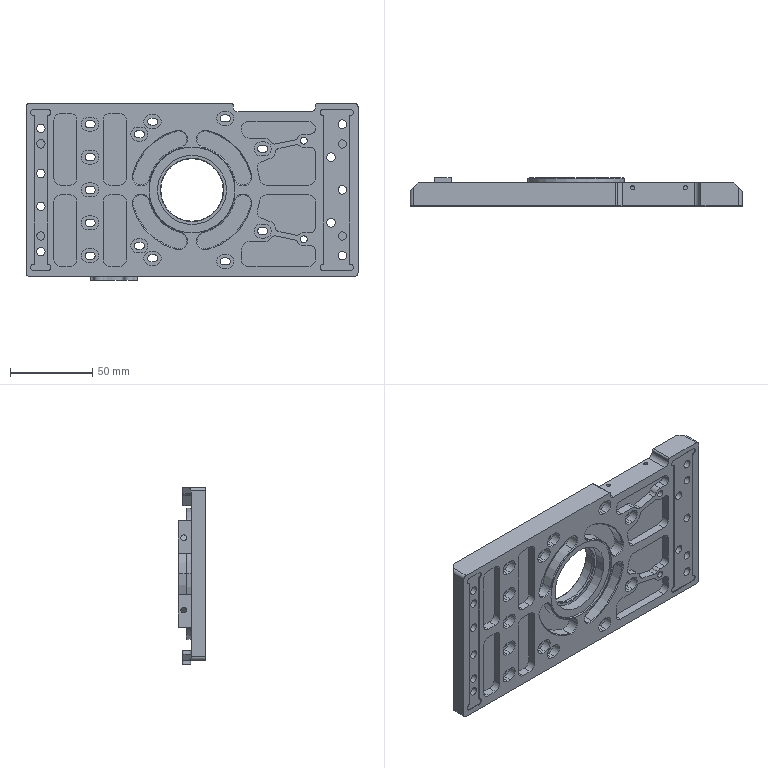NC program | Mastercam | posted with a generic post | part box 202 x 17 x 107.5 mm
Lines 37 to 829 of 36425:
(10 FEM |TOOL - 10|DIA. OFF. - 10|LEN. - 10|TOOL DIA. - 10.)
N140 T10 M6
N142 G0 G54 G90 X-108.252 Y-63.233 C0. B0. S8000 M3
N144 G43 H10 Z30.
N146 Z1.
N148 G1 Z-16.55 F600.
N150 X-108.566 Y-62.39 Z-16.671 F3000.
N152 G3 X-109.084 Y-61.584 Z-16.8 I-2.109 J-.785
N154 G2 X-109.891 Y-60.208 I8.129 J5.7
N156 X-110.45 Y-58.241 I6.899 J3.023
N158 X-110.619 Y-55.793 I17.678 J2.448
N160 G1 Y-55.785
N162 G2 X-110.56 Y-46.813 I903.244 J-1.493
N164 G1 X-110.556 Y-46.425
N166 X-110.202 Y-7.338
N168 X-109.983 Y18.252
N170 X-109.968 Y55.318
N172 G2 X-108.458 Y59.085 I5.565 J-.044
N174 X-106.071 Y60.843 I5.756 J-5.316
N176 X-102.937 Y61.864 I5.496 J-11.553
N178 X-98.831 Y62.325 I5.277 J-28.453
N180 X-92.414 Y62.461 I6.417 J-151.176
N182 G1 X-92.254
N184 G2 X-88.645 Y62.471 I4.557 J-985.763
N186 G1 X-88.244 Y62.472
N188 X-48.292 Y62.475
N190 X-8.345
N192 X31.603
N194 X71.55
N196 X102.839 Y62.467
N198 G2 X106.602 Y60.942 I-.064 J-5.565
N200 X108.352 Y58.553 I-5.351 J-5.753
N202 X109.367 Y55.42 I-11.605 J-5.492
N204 X109.826 Y51.316 I-28.581 J-5.274
N206 X109.961 Y44.9 I-151.93 J-6.416
N208 G1 Y44.741
N210 G2 X109.971 Y41.131 I-990.762 J-4.557
N212 G1 X109.972 Y40.731
N214 X109.975 Y.779
N216 Y-39.169
N218 X109.97 Y-55.246
N220 G2 X109.609 Y-57.242 I-5.984 J.054
N222 X107.77 Y-59.746 I-5.807 J2.336
N224 X105.594 Y-61.063 I-5.496 J6.626
N226 X102.506 Y-61.944 I-5.363 J12.94
N228 X98.455 Y-62.344 I-5.194 J31.922
N230 X91.898 Y-62.465 I-6.557 J177.511
N232 G1 X91.499
N234 G2 X89.493 Y-62.47 I-3.687 J993.144
N236 G1 X89.093 Y-62.471
N238 X49.139 Y-62.475
N240 X9.192
N242 X-30.756
N244 X-70.703
N246 X-102.779 Y-62.469
N248 G2 X-106.004 Y-61.272 I.254 J5.626
N250 X-108.106 Y-58.694 I4.657 J5.944
N252 X-109.126 Y-55.777 I10.611 J5.347
N254 X-109.605 Y-52.037 I24.378 J5.02
N256 X-109.733 Y-46.949 I101.295 J5.088
N258 X-109.73 Y-46.207 I101.423
N260 X-109.687 Y-38.984 I979.503 J-2.141
N262 G1 X-109.684 Y-38.584
N264 X-109.324 Y1.364
N266 X-109.187 Y18.119
N268 X-109.169 Y52.967
N270 G2 X-107.095 Y57.857 I7.26 J-.195
N272 X-104.615 Y59.685 I6.688 J-6.48
N274 X-101.097 Y60.906 I6.323 J-12.532
N276 X-97.002 Y61.447 I5.83 J-28.342
N278 X-90.78 Y61.644 I6.522 J-107.624
N280 X-83.161 Y61.673 I7.619 J-998.469
N282 G1 X-82.354
N284 X-81.954
N286 X-42.004 Y61.675
N288 X-2.057
N290 X37.891
N292 X77.838
N294 X100.549 Y61.666
N296 G2 X105.417 Y59.537 I-.281 J-7.272
N298 X107.219 Y57.048 I-6.596 J-6.672
N300 X108.42 Y53.534 I-12.702 J-6.303
N302 X108.951 Y49.445 I-28.74 J-5.816
N304 X109.145 Y43.227 I-109.36 J-6.516
N306 X109.173 Y35.78 I-984.996 J-7.447
N308 G1 Y35.201
N310 Y34.801
N312 X109.175 Y-5.149
N314 Y-45.096
N316 X109.167 Y-53.013
N318 G2 X107.062 Y-57.891 I-7.264 J.242
N320 X104.577 Y-59.704 I-6.679 J6.545
N322 X101.062 Y-60.914 I-6.311 J12.627
N324 X96.97 Y-61.45 I-5.822 J28.564
N326 X90.75 Y-61.645 I-6.519 J108.595
N328 X83.302 Y-61.673 I-7.448 J977.606
N330 G1 X82.724
N332 X82.324
N334 X42.374 Y-61.675
N336 X2.427
N338 X-37.521
N340 X-77.468
N342 X-100.397 Y-61.664
N344 G2 X-105.252 Y-59.529 I.322 J7.317
N346 X-107.055 Y-57.034 I6.568 J6.647
N348 X-108.247 Y-53.507 I12.593 J6.221
N350 X-108.754 Y-49.406 I28.302 J5.58
N352 X-108.898 Y-43.847 I107.126 J5.559
N354 X-108.896 Y-43.181 I107.27
N356 X-108.849 Y-34.755 I989.918 J-1.341
N358 G1 X-108.845 Y-34.355
N360 X-108.485 Y5.593
N362 X-108.389 Y18.354
N364 X-108.366 Y50.809
N366 G2 X-107.672 Y54.161 I8.943 J-.105
N368 X-105.173 Y57.445 I8.034 J-3.521
N370 X-101.736 Y59.371 I7.364 J-9.11
N372 X-97.917 Y60.311 I6.593 J-18.555
N374 X-92.713 Y60.746 I6.575 J-47.295
N376 X-84.724 Y60.866 I7.989 J-265.907
N378 G1 X-84.189 Y60.865
N380 X-83.788 Y60.867
N382 X-43.83 Y60.875
N384 X-3.882
N386 X36.065
N388 X76.012
N390 X98.037 Y60.872
N392 X98.078
N394 G2 X100.704 Y60.514 J-9.808
N396 X104.928 Y57.693 I-2.463 J-8.261
N398 X106.862 Y54.259 I-9.072 J-7.372
N400 X107.808 Y50.438 I-18.476 J-6.599
N402 X108.245 Y45.232 I-47.073 J-6.579
N404 X108.366 Y37.242 I-264.495 J-7.99
N406 G1 X108.365 Y36.707
N408 X108.367 Y36.306
N410 X108.375 Y-3.652
N412 Y-43.599
N414 X108.373 Y-50.427
N416 G2 X108.374 Y-50.532 I-10.151 J-.105
N418 X108.054 Y-53.06 I-10.152
N420 X105.3 Y-57.337 I-8.263 J2.294
N422 X102.118 Y-59.224 I-7.277 J8.649
N424 X98.27 Y-60.255 I-6.695 J17.287
N426 X93.454 Y-60.715 I-6.357 J41.134
N428 X85.886 Y-60.86 I-7.568 J197.068
N430 G1 X85.702
N432 G2 X83.295 Y-60.868 I-4.457 J977.996
N434 G1 X82.894 Y-60.869
N436 X42.939 Y-60.875
N438 X2.992
N440 X-36.956
N442 X-76.903
N444 X-97.709 Y-60.873
N446 G2 X-97.827 Y-60.874 I-.118 J10.384
N448 X-100.324 Y-60.569 J10.385
N450 X-104.626 Y-57.844 I2.209 J8.246
N452 X-106.529 Y-54.655 I8.508 J7.238
N454 X-107.556 Y-50.789 I16.984 J6.58
N456 X-107.986 Y-45.959 I40.193 J6.017
N458 X-108.075 Y-40.112 I191.325 J5.847
N460 X-108.066 Y-38.2 I191.414
N462 X-108.05 Y-35.393 I981.197 J-4.278
N464 G1 X-108.047 Y-34.993
N466 X-107.691 Y4.96
N468 X-107.591 Y18.52
N470 X-107.57 Y48.519
N472 G2 X-107.304 Y51.205 I13.756 J-.009
N474 X-104.319 Y56.213 I9.035 J-1.992
N476 X-100.98 Y58.251 I7.766 J-8.966
N478 X-97.164 Y59.338 I7.048 J-17.505
N480 X-92.33 Y59.866 I6.695 J-38.843
N482 X-84.95 Y60.05 I7.663 J-159.972
N484 X-79.333 Y60.07 I6.399 J-975.619
N486 G1 X-78.933 Y60.071
N488 X-38.981 Y60.075
N490 X.967
N492 X40.914
N494 X80.862
N496 X96.104 Y60.069
N498 G2 X98.815 Y59.779 I-.049 J-13.268
N500 X103.585 Y56.961 I-2.09 J-8.985
N502 X105.685 Y53.637 I-8.68 J-7.807
N504 X106.81 Y49.813 I-17.037 J-7.09
N506 X107.359 Y44.966 I-37.713 J-6.723
N508 X107.549 Y37.58 I-154.608 J-7.674
N510 X107.571 Y31.562 I-969.556 J-6.559
N512 G1 Y31.162
N514 X107.575 Y-8.79
N516 X107.564 Y-48.834
N518 G2 X107.204 Y-51.615 I-11.6 J.089
N520 X104.462 Y-56.084 I-8.928 J2.401
N522 X101.137 Y-58.185 I-7.807 J8.677
N524 X97.312 Y-59.31 I-7.091 J17.037
N526 X92.465 Y-59.859 I-6.722 J37.715
N528 X85.079 Y-60.049 I-7.673 J154.619
N530 X79.062 Y-60.071 I-6.558 J969.621
N532 G1 X78.662
N534 X38.71 Y-60.075
N536 X-1.238
N538 X-41.185
N540 X-81.133
N542 X-95.984 Y-60.068
N544 X-95.985
N546 G2 X-98.718 Y-59.76 J12.293
N548 X-103.466 Y-56.897 I2.165 J8.957
N550 X-105.533 Y-53.552 I8.765 J7.729
N552 X-106.622 Y-49.719 I17.127 J6.936
N554 X-107.126 Y-44.868 I37.817 J6.381
N556 X-107.253 Y-38.594 I154.788 J6.274
N558 X-107.249 Y-37.48 I154.915
N560 X-107.216 Y-31.463 I969.645 J-2.216
N562 G1 X-107.213 Y-31.063
N564 X-106.856 Y8.886
N566 X-106.786 Y21.244
N568 X-106.766 Y46.871
N570 G2 X-106.551 Y49.424 I17.004 J-.145
N572 X-106.152 Y50.983 I10.119 J-1.762
N574 G3 X-106.123 Y51.121 I-.569 J.19
N576 G2 X-101.185 Y57.308 I7.123 J-.621
N578 X-94.561 Y58.766 I9.905 J-29.216
N580 X-88.242 Y59.168 I7.744 J-71.873
N582 X-78.476 Y59.271 I9.766 J-463.902
N584 X-77.354 Y59.27 J-464.005
N586 G1 X-76.954
N588 X-37.001 Y59.275
N590 X2.946
N592 X42.894
N594 X82.841
N596 X94.513 Y59.263
N598 G2 X97.099 Y59.019 I-.211 J-16.032
N600 X100.898 Y57.425 I-1.8 J-9.617
N602 G3 X101.064 Y57.346 I.339 J.495
N604 G2 X106.146 Y50.732 I-2.064 J-6.846
N606 G3 X106.388 Y47.256 I115.254 J6.278
N608 G2 X106.731 Y37.844 I-150.383 J-10.187
N610 X106.772 Y29.06 I-947.064 J-8.784
N612 G1 Y28.615
N614 Y28.215
N616 X106.775 Y-11.736
N618 X106.764 Y-46.972
N620 G2 X106.529 Y-49.546 I-16.28 J.189
N622 X106.15 Y-50.988 I-10.095 J1.879
N624 G3 X106.123 Y-51.122 I.571 J-.186
N626 G2 X101.184 Y-57.308 I-7.123 J.622
N628 X94.56 Y-58.767 I-9.904 J29.216
N630 X88.241 Y-59.168 I-7.744 J71.887
N632 X78.475 Y-59.271 I-9.766 J464.022
N634 X77.353 Y-59.27 J464.125
N636 G1 X76.953
N638 X37. Y-59.275
N640 X-2.947
N642 X-42.895
N644 X-82.842
N646 X-94.089 Y-59.267
N648 G2 X-96.608 Y-59.075 I.098 J17.869
N650 X-100.601 Y-57.506 I1.517 J9.728
N652 G3 X-100.786 Y-57.423 I-.335 J-.498
N654 G2 X-106.15 Y-50.5 I1.786 J6.923
N656 G1 Y-50.101
N658 G3 X-106.267 Y-46.263 I-84.646 J-.654
N660 G2 X-106.442 Y-37.306 I229.01 J8.957
N662 X-106.433 Y-35.307 I229.185
N664 X-106.414 Y-31.697 I987.932 J-3.31
N666 G1 X-106.412 Y-31.297
N668 X-106.15 Y-1.572
N670 G3 X-106.149 Y-1.168 I-89.012 J.404
N672 X-106.15 Y-.768 I-89.013
N674 G1 Y-.369
N676 Y39.579
N678 Y50.5
N680 G2 X-106.05 Y51.693 I7.15
N682 G3 X-106.019 Y52.068 Z-16.75 I-2.218 J.375
N684 X-106.505 Y53.466 Z-16.55 I-2.249
N686 X-108.268 Y54.318 I-1.763 J-1.398 F9999.
N688 X-110.518 Y52.071 J-2.25
N690 G1 X-110.65 Y-50.297
N692 Y-50.3
N694 G3 X-108.4 Y-52.55 I2.25
N696 X-106.894 Y-51.972 J2.25
N698 X-106.15 Y-50.3 Z-16.8 I-1.506 J1.672 F3000.
N700 G1 Y-49.701
N702 Y-9.754
N704 Y-.965
N706 G3 X-106.354 Y-.029 Z-16.672 I-2.25
N708 G1 X-106.737 Y.807 Z-16.55
N710 X-106.966 Y1.309 F9999.
N712 G3 X-109.039 Y2.64 I-2.073 J-.948
N714 X-111.318 Y.361 J-2.279
N716 X-111.313 Y.213 I2.279
N718 G1 X-108.21 Y-47.426
N720 G3 X-92.618 Y-62.036 I15.592 J1.015
N722 G1 X-92.572
N724 X104.51 Y-61.463
N726 G3 X106.737 Y-59.229 I-.007 J2.234
N728 X104.581 Y-56.996 I-2.234
N730 G1 X103.656 Y-56.964
N732 X103.608 Y-56.962
N734 X102.69 Y-56.93 Z-16.672 F3000.
N736 G3 X102.611 Y-56.929 Z-16.682 I-.079 J-2.249
N738 X101.747 Y-57.101 Z-16.8 J-2.25
N740 G2 X98.915 Y-57.657 I-2.832 J6.935
N742 X98.693 Y-57.654 J7.491
N744 G3 X95.765 Y-57.87 I2.336 J-51.552
N746 G2 X85.109 Y-58.409 I-11.815 J127.926
N748 X73.727 Y-58.474 I-11.382 J991.428
N750 X71.865 Y-58.473 J991.493
N752 G1 X71.466
N754 X31.516 Y-58.475
N756 X-8.431
N758 X-48.379
N760 X-88.326
N762 G2 X-89.317 Y-58.476 I-.991 J329.874
N764 X-92.816 Y-58.458 J329.875
N766 X-95.858 Y-58.145 I.186 J16.743
N768 X-97.513 Y-57.68 I3.473 J15.545
N770 G3 X-97.701 Y-57.65 I-.188 J-.57
N772 G1 X-98.1
N774 G2 X-98.5 Y-57.653 I-.4 J29.026
N776 X-99.399 Y-57.639 J29.029
N778 X-101.352 Y-57.252 I.399 J7.139
N780 G3 X-102.092 Y-57.127 Z-16.7 I-.74 J-2.125
N782 X-103.176 Y-57.405 Z-16.55 J-2.25
N784 X-104.342 Y-59.377 I1.084 J-1.972 F9999.
N786 X-102.098 Y-61.627 I2.25
N788 G1 X99.764 Y-62.118
N790 X99.77
N792 G3 X102.02 Y-59.868 J2.25
N794 X101.313 Y-58.231 I-2.25
N796 X99.77 Y-57.618 Z-16.776 I-1.543 J-1.637 F3000.
N798 X99.586 Y-57.626 Z-16.8 J-2.25
N800 G2 X98.59 Y-57.655 I-.996 J17.242
N802 X98.188 Y-57.65 J17.271
N804 G1 X97.789
N806 X76.222 Y-57.667
N808 X36.268 Y-57.675
N810 X-3.68
N812 X-43.627
N814 X-83.574
N816 G2 X-85.372 Y-57.677 I-1.798 J854.826
N818 X-91.256 Y-57.657 J854.828
N820 G3 X-95.107 Y-57.649 I-3.851 J-926.097
N822 X-96.705 Y-57.65 J-926.105
N824 G1 X-97.104
N826 X-98.302
N828 G3 X-99.975 Y-58.394 Z-16.55 J-2.25
N830 X-100.553 Y-59.9 I1.673 J-1.506 F9999.
N832 X-98.302 Y-62.15 I2.251
N834 G1 X84.31
N836 G3 X86.56 Y-59.9 J2.25
N838 X85.982 Y-58.394 I-2.25
N840 X84.31 Y-57.65 Z-16.8 I-1.672 J-1.506 F3000.
N842 G1 X83.711
N844 X43.763
N846 X3.816
N848 X-36.132
N850 X-76.079
N852 X-92.058
N854 G3 X-92.994 Y-57.854 Z-16.672 J-2.25
N856 G1 X-93.83 Y-58.237 Z-16.55
N858 X-94.332 Y-58.467 F9999.
N860 G2 X-98.338 Y-59.34 I-4.006 J8.753
N862 X-107.964 Y-49.768 J9.626
N864 G1 X-108.538 Y52.223
N866 Y52.25
N868 G2 X-103.821 Y56.967 I4.717
N870 X-103.609 Y56.962 J-4.717
N872 G1 X-102.69 Y56.93 Z-16.672 F3000.
N874 G3 X-102.612 Y56.929 Z-16.682 I.078 J2.248
N876 X-101.747 Y57.101 Z-16.8 J2.249
N878 G2 X-98.915 Y57.657 I2.832 J-6.934
N880 X-98.693 Y57.654 J-7.49
N882 G3 X-95.765 Y57.87 I-2.336 J51.552
N884 G2 X-85.109 Y58.409 I11.815 J-127.925
N886 X-73.726 Y58.474 I11.383 J-991.557
N888 X-71.865 Y58.473 J-991.622
N890 G1 X-71.466
N892 X-31.516 Y58.475
N894 X8.431
N896 X48.379
N898 X88.326
N900 G2 X89.514 Y58.478 I1.188 J-256.285
N902 X93.246 Y58.451 J-256.288
N904 X96.343 Y58.075 I-.299 J-15.42
N906 X97.674 Y57.68 I-3.568 J-14.485
N908 G3 X97.863 Y57.65 I.189 J.57
N910 G1 X98.263
N912 G2 X98.691 Y57.658 I.428 J-11.703
N914 X99.797 Y57.605 J-11.711
N916 X101.352 Y57.252 I-.797 J-7.105
N918 G3 X102.092 Y57.127 Z-16.7 I.74 J2.125
N920 X102.304 Y57.137 Z-16.672 J2.25
N922 G1 X103.219 Y57.223 Z-16.55
N924 X103.267 Y57.228 F9999.
N926 G2 X103.478 Y57.238 I.211 J-2.241
N928 X105.233 Y56.395 J-2.251
N930 G1 X106.108 Y55.304
N932 G2 X106.603 Y53.895 I-1.757 J-1.409
N934 X106.479 Y53.157 I-2.252
N936 G1 X106.196 Y52.283 Z-16.672 F3000.
N938 G3 X106.087 Y51.59 Z-16.765 I2.141 J-.693
N940 X106.102 Y51.329 Z-16.8 I2.25
N942 G2 X106.154 Y50.358 I-9.059 J-.971
N944 X106.15 Y50.101 I-9.111
N946 G1 Y49.701
N948 Y9.754
N950 Y-30.194
N952 Y-50.5
N954 G2 X106.05 Y-51.693 I-7.15
N956 G3 X106.019 Y-52.068 Z-16.75 I2.218 J-.375
N958 X106.095 Y-52.65 Z-16.672 I2.249
N960 G1 X106.333 Y-53.538 Z-16.55
N962 X106.345 Y-53.585 F9999.
N964 G2 X106.489 Y-54.682 I-4.099 J-1.097
N966 X102.287 Y-58.925 I-4.243
N968 G1 X-98.914 Y-60.859
N970 X-98.998
N972 G2 X-107.658 Y-52.199 J8.66
N974 G1 Y-52.196
N976 X-107.613 Y53.757
N978 G2 X-103.011 Y58.357 I4.602 J-.002
N980 X-101.4 Y58.066 J-4.602
N982 G1 X-100.536 Y57.753 Z-16.672 F3000.
N984 G3 X-99.77 Y57.619 Z-16.776 I.766 J2.115
N986 X-99.586 Y57.626 Z-16.8 J2.249
N988 G2 X-98.59 Y57.655 I.996 J-17.242
N990 X-98.188 Y57.65 J-17.271
N992 G1 X-97.789
N994 X-76.222 Y57.667
N996 X-36.268 Y57.675
N998 X3.68
N1000 X43.627
N1002 X83.574
N1004 X91.239 Y57.661
N1006 G3 X95.883 Y57.648 I4.644 J854.329
N1008 X97.681 Y57.65 J854.342
N1010 G1 X98.08
N1012 X98.48
N1014 G3 X100.152 Y58.394 Z-16.55 J2.25
N1016 X100.73 Y59.9 I-1.672 J1.506 F9999.
N1018 X98.48 Y62.15 I-2.25
N1020 G1 X-84.31
N1022 G3 X-86.56 Y59.9 J-2.25
N1024 X-85.982 Y58.394 I2.25
N1026 X-84.31 Y57.65 Z-16.8 I1.672 J1.506 F3000.
N1028 G1 X-83.711
N1030 X-43.763
N1032 X-3.816
N1034 X24.
N1036 G2 X25.866 Y57.372 I-.039 J-6.664
N1038 G3 X28.396 Y57.049 I3.448 J16.959
N1040 X33.749 Y56.898 I5.466 J98.541
N1042 X40.094 Y56.877 I6.345 J945.228
N1044 G1 X40.509
N1046 X40.908
N1048 X72.86 Y56.875
N1050 G3 X73.139 Y56.944 J.6
N1052 G2 X76. Y57.65 I2.861 J-5.444
N1054 G1 X76.399
N1056 X92.378
N1058 G3 X94.051 Y58.394 Z-16.55 J2.25
N1060 X94.629 Y59.9 I-1.673 J1.506 F9999.
N1062 X92.378 Y62.151 I-2.251
N1064 G1 X92.374
N1066 X25.421 Y62.028
N1068 G3 X23.175 Y59.778 I.004 J-2.25
N1070 X23.522 Y58.578 I2.25
N1072 X25.043 Y57.561 Z-16.8 I1.903 J1.2 F3000.
N1074 G2 X26.745 Y57.003 I-1.043 J-6.061
N1076 G3 X28.536 Y56.539 I2.993 J7.86
N1078 X32.034 Y56.214 I4.599 J30.518
N1080 X39.023 Y56.086 I6.989 J190.354
N1082 X39.452 Y56.087 J190.482
N1084 X41.044 Y56.082 I3.791 J990.721
N1086 G1 X41.442 Y56.081
N1088 X70.909 Y56.08
N1090 G3 X71.809 Y56.138 I-.098 J8.508
N1092 X72.117 Y56.269 I-.071 J.596
N1094 G2 X73.472 Y57.106 I3.883 J-4.769
N1096 G3 X74.69 Y58.472 Z-16.55 I-.925 J2.052
N1098 X74.797 Y59.158 I-2.143 J.686 F9999.
N1100 X72.557 Y61.408 I-2.25
N1102 G1 X27.01 Y61.596
N1104 X27.001
N1106 G3 X24.751 Y59.346 J-2.25
N1108 X24.901 Y58.537 I2.25
N1110 X26.197 Y57.244 Z-16.8 I2.1 J.809 F3000.
N1112 G2 X27.435 Y56.601 I-2.197 J-5.744
N1114 G3 X28.961 Y56.031 I2.875 J5.364
N1116 X32.231 Y55.542 I4.666 J20.025
N1118 X37.946 Y55.321 I6.231 J87.112
N1120 X47.479 Y55.275 I9.533 J990.993
N1122 X49.077 Y55.276 J991.039
N1124 G1 X49.477
N1126 X69.36 Y55.286
N1128 X69.4
N1130 G3 X70.988 Y55.424 J9.191
N1132 G1 X71.141 Y55.459
N1134 G3 X71.452 Y55.64 I-.132 J.585
N1136 G2 X72.34 Y56.442 I4.548 J-4.14
N1138 G3 X73.241 Y58.036 Z-16.55 I-1.339 J1.809
N1140 X73.251 Y58.251 I-2.24 J.215 F9999.
N1142 X71.035 Y60.5 I-2.25
N1144 G1 X28.026 Y61.141
N1146 X27.992
N1148 G3 X25.742 Y58.891 J-2.25
N1150 X25.805 Y58.361 I2.25
N1152 X26.923 Y56.911 Z-16.8 I2.187 J.53 F3000.
N1154 G2 X28.022 Y56.153 I-2.923 J-5.411
N1156 G3 X29.41 Y55.506 I2.901 J4.414
N1158 X32.169 Y54.927 I4.498 J14.566
N1160 X36.961 Y54.59 I5.949 J50.336
N1162 X45.682 Y54.482 I8.721 J351.081
N1164 G1 X46.426
N1166 X46.824 Y54.481
N1168 X67.539 Y54.483
N1170 X67.55
N1172 G3 X69.798 Y54.613 J19.467
N1174 X70.679 Y54.821 I-.571 J4.401
N1176 X70.972 Y55.042 I-.197 J.566
N1178 G2 X71.753 Y55.948 I5.028 J-3.542
N1180 G3 X72.449 Y57.575 Z-16.559 I-1.554 J1.627
N1182 X72.448 Y57.641 Z-16.55 I-2.25
N1184 X70.242 Y59.825 I-2.249 J-.066 F9999.
N1186 G1 X28.892 Y60.609
N1188 X28.849
N1190 G3 X26.599 Y58.359 J-2.25
N1192 X26.615 Y58.095 I2.25
N1194 X27.55 Y56.522 Z-16.8 I2.234 J.264 F3000.
N1196 G2 X28.506 Y55.702 I-4.852 J-6.628
N1198 G3 X29.759 Y54.998 I2.924 J3.736
N1200 X32.369 Y54.306 I4.556 J11.905
N1202 X36.668 Y53.874 I5.945 J37.545
N1204 X44.47 Y53.698 I7.958 J180.566
N1206 X48.846 Y53.682 I5.825 J955.241
N1208 G1 X49.244 Y53.681
N1210 X65.973 Y53.683
N1212 X66.055
N1214 G3 X68.726 Y53.816 J26.873
N1216 X70.091 Y54.107 I-.58 J6.072
N1218 X70.334 Y54.208 I-.988 J2.705
N1220 X70.612 Y54.466 I-.247 J.547
N1222 G2 X71.289 Y55.453 I5.388 J-2.966
N1224 G3 X71.815 Y56.899 Z-16.592 I-1.724 J1.446
N1226 X71.793 Y57.212 Z-16.55 I-2.25
N1228 X69.622 Y59.148 I-2.228 J-.313 F9999.
N1230 G1 X29.474 Y60.169
N1232 G3 X29.417 Y60.17 I-.057 J-2.249
N1234 X27.167 Y57.92 J-2.25
N1236 X27.168 Y57.847 I2.25
N1238 X27.966 Y56.2 Z-16.8 I2.249 J.073 F3000.
N1240 G2 X28.806 Y55.337 I-3.966 J-4.7
N1242 G3 X29.858 Y54.59 I2.66 J2.627
N1244 X32.257 Y53.762 I4.504 J9.166
N1246 X36.403 Y53.184 I6.052 J28.235
N1248 X42.938 Y52.932 I7.386 J107.043
N1250 X53.589 Y52.875 I10.651 J997.794
N1252 X55.265 Y52.877 J997.851
N1254 G1 X55.664
N1256 X64.802 Y52.886
N1258 G3 X67.955 Y53.045 I-.018 J31.745
N1260 X69.658 Y53.42 I-.786 J7.629
N1262 X70.077 Y53.618 I-1.059 J2.783
N1264 X70.342 Y53.909 I-.287 J.526
N1266 G2 X70.915 Y54.959 I5.658 J-2.409
N1268 G3 X71.305 Y56.225 Z-16.622 I-1.86 J1.266
N1270 X71.24 Y56.761 Z-16.55 I-2.25
N1272 X69.12 Y58.474 I-2.185 J-.536 F9999.
N1274 G1 X30.088 Y59.604
N1276 G3 X30.023 Y59.605 I-.065 J-2.249
N1278 X27.778 Y57.505 J-2.25
N1280 X27.773 Y57.355 Z-16.57 I2.245 J-.15 F3000.
N1282 X28.41 Y55.787 Z-16.8 I2.25
N1284 G2 X29.147 Y54.879 I-5.548 J-5.263
N1286 G3 X30.121 Y54.093 I2.673 J2.313
N1288 X32.408 Y53.177 I4.57 J8.1
N1290 X35.122 Y52.65 I5.175 J19.399
N1292 G1 X35.521
N1294 X68.109 Y52.657
N1296 G3 X69.64 Y52.987 I-.162 J4.47
N1298 X69.918 Y53.137 I-.897 J1.994
N1300 X70.169 Y53.456 I-.318 J.509
N1302 G2 X70.472 Y54.194 I5.831 J-1.956
N1304 G3 X70.699 Y55.18 Z-16.665 I-2.023 J.986
N1306 X70.535 Y56.024 Z-16.55 I-2.25
N1308 X68.449 Y57.43 I-2.086 J-.844 F9999.
N1310 X67.925 Y57.368 J-2.25
N1312 G1 X66.755 Y57.088
N1314 G3 X65.029 Y54.9 I.524 J-2.188
N1316 X65.607 Y53.394 I2.25
N1318 X67.279 Y52.65 Z-16.8 I1.672 J1.506 F3000.
N1320 G1 X67.879
N1322 X69.191 Y52.657
N1324 G3 X69.768 Y52.814 I-.125 J1.594
N1326 X70.087 Y53.191 I-.258 J.542
N1328 G2 X70.356 Y53.943 I5.913 J-1.691
N1330 G3 X70.507 Y54.673 Z-16.7 I-1.686 J.73
N1332 X70.168 Y55.737 Z-16.55 I-1.837
N1334 X68.67 Y56.51 I-1.498 J-1.064 F9999.
N1336 X67.393 Y55.994 J-1.837
N1338 G1 X67.201 Y55.809
N1340 G3 X66.64 Y54.487 I1.277 J-1.322
N1342 X66.906 Y53.535 I1.838
N1344 X68.478 Y52.65 Z-16.8 I1.572 J.952 F3000.
N1346 G1 X69.077
N1348 X69.481
N1350 G3 X70.06 Y53.094 J.6
N1352 G2 X70.176 Y53.477 I5.94 J-1.594
N1354 G3 X70.295 Y54.2 Z-16.702 I-2.13 J.723
N1356 X70.009 Y55.299 Z-16.55 I-2.249
N1358 X68.206 Y56.444 I-1.963 J-1.099 F9999.
N1360 G1 X30.603 Y59.135
N1362 G3 X30.442 Y59.141 I-.161 J-2.244
N1364 X28.214 Y57.207 J-2.25
N1366 X28.192 Y56.891 Z-16.592 I2.228 J-.316 F3000.
N1368 X28.717 Y55.447 Z-16.8 I2.25
N1370 G2 X29.424 Y54.423 I-6.254 J-5.077
N1372 G3 X30.536 Y53.472 I2.934 J2.306
N1374 X32.284 Y52.682 I4.55 J7.741
N1376 X32.478 Y52.65 I.194 J.568
N1378 G1 X32.877
N1380 X35.674
N1382 G3 X37.346 Y53.394 Z-16.55 J2.25
N1384 X37.924 Y54.9 I-1.672 J1.506 F9999.
N1386 X36.311 Y57.058 I-2.25
N1388 G1 X31.52 Y58.473
N1390 G3 X30.883 Y58.565 I-.637 J-2.158
N1392 X28.691 Y56.822 J-2.25
N1394 X28.633 Y56.315 Z-16.618 I2.192 J-.507 F3000.
N1396 X29.039 Y55.025 Z-16.8 I2.25
N1398 G2 X29.596 Y54.063 I-6.138 J-4.192
N1400 G3 X30.524 Y53.1 I2.982 J1.944
N1402 X31.109 Y52.724 I3.096 J4.184
N1404 X31.398 Y52.65 I.289 J.526
N1406 G1 X31.798
N1408 X32.996
N1410 G3 X34.668 Y53.394 Z-16.55 J2.25
N1412 X35.246 Y54.9 I-1.672 J1.506 F9999.
N1414 X34.036 Y56.895 I-2.25
N1416 G1 X32.232 Y57.836
N1418 G3 X31.192 Y58.091 I-1.04 J-1.995
N1420 X29.039 Y56.494 J-2.25
N1422 X28.942 Y55.841 Z-16.638 I2.153 J-.653 F3000.
N1424 X29.265 Y54.678 Z-16.8 I2.25
N1426 G2 X29.783 Y53.617 I-6.901 J-4.024
N1428 G3 X30.49 Y52.78 I2.333 J1.254
N1430 X30.863 Y52.65 I.373 J.47
N1432 G1 X31.262
N1434 X32.061
N1436 G3 X33.733 Y53.394 Z-16.55 J2.25
N1438 X34.311 Y54.9 I-1.672 J1.506 F9999.
N1440 X33.303 Y56.777 I-2.25
N1442 G1 X32.75 Y57.142
N1444 G3 X31.509 Y57.515 I-1.241 J-1.877
N1446 X29.413 Y56.085 J-2.25
N1448 X29.258 Y55.265 Z-16.661 I2.096 J-.82 F3000.
N1450 X29.497 Y54.257 Z-16.8 I2.251
N1452 G2 X29.9 Y53.252 I-6.177 J-3.057
N1454 G3 X30.131 Y52.871 I1.293 J.522
N1456 X30.596 Y52.65 I.465 J.379
N1458 G1 X30.995
N1460 X31.395
N1462 G3 X32.966 Y53.535 Z-16.55 J1.837
N1464 X33.232 Y54.487 I-1.571 J.952 F9999.
N1466 X33.152 Y55.025 I-1.837
N1468 X31.36 Y56.448 I-1.792 J-.417
N1470 X29.868 Y55.686 J-1.84
N1472 X29.52 Y54.61 Z-16.703 I1.489 J-1.076 F3000.
N1474 X29.665 Y53.894 Z-16.8 I1.837
N1476 G2 X29.94 Y53.094 I-5.665 J-2.394
N1478 G3 X30.519 Y52.65 I.579 J.156
N1480 G1 X30.919
N1482 X31.318
N1484 G3 X32.255 Y52.854 Z-16.672 J2.25
N1486 G1 X33.09 Y53.237 Z-16.55
N1488 X33.592 Y53.467 F9999.
N1490 G0 Z30.
N1492 S6500 M3
N1494 Z50.
N1496 X6.351 Y-1.569
N1498 Z4.279
N1500 G1 Z3.779 F600.
N1502 X6.33 Y-1.493 Z3.222
N1504 X6.269 Y-1.271 Z2.71
N1506 X6.172 Y-.92 Z2.282
N1508 X6.047 Y-.468 Z1.972
N1510 X5.905 Y.049 Z1.805
N1512 X5.695 Y.753 Z1.706
N1514 X5.297 Y1.63 Z1.536
N1516 X4.757 Y2.427 Z1.366
N1518 X4.091 Y3.123 Z1.196
N1520 X3.317 Y3.696 Z1.026
N1522 X2.458 Y4.13 Z.856
N1524 X1.537 Y4.414 Z.686
N1526 X.582 Y4.539 Z.516
N1528 X-.38 Y4.501 Z.346
N1530 X-1.19 Y4.34 Z.2
N1532 X-1.987 Y4.036 Z.193 F2000.
N1534 X-2.713 Y3.587 Z.185
N1536 X-3.341 Y3.01 Z.178
N1538 X-3.848 Y2.324 Z.17
N1540 X-4.218 Y1.555 Z.163
N1542 X-4.435 Y.73 Z.155
N1544 X-4.493 Y-.121 Z.148
N1546 X-4.389 Y-.966 Z.14
N1548 X-4.128 Y-1.777 Z.133
N1550 X-3.719 Y-2.524 Z.125
N1552 X-3.176 Y-3.181 Z.118
N1554 X-2.52 Y-3.723 Z.111
N1556 X-1.773 Y-4.132 Z.103
N1558 X-.962 Y-4.393 Z.096
N1560 X-.116 Y-4.497 Z.088
N1562 X.734 Y-4.439 Z.081
N1564 X1.557 Y-4.223 Z.073
N1566 X2.325 Y-3.855 Z.066
N1568 X3.011 Y-3.348 Z.058
N1570 X3.588 Y-2.722 Z.051
N1572 X4.037 Y-1.998 Z.044
N1574 X4.341 Y-1.203 Z.036
N1576 X4.491 Y-.364 Z.029
N1578 X4.479 Y.488 Z.021
N1580 X4.307 Y1.322 Z.014
N1582 X3.981 Y2.109 Z.006
N1584 X3.513 Y2.821 Z-.001
N1586 X2.919 Y3.431 Z-.009
N1588 X2.22 Y3.919 Z-.016
N1590 X1.442 Y4.266 Z-.023
N1592 X.613 Y4.46 Z-.031
N1594 X-.238 Y4.495 Z-.038
N1596 X-1.081 Y4.368 Z-.046
N1598 X-1.884 Y4.085 Z-.053
N1600 X-2.62 Y3.656 Z-.061
N1602 X-3.261 Y3.096 Z-.068
N1604 X-3.786 Y2.425 Z-.076
N1606 X-4.175 Y1.667 Z-.083
N1608 X-4.414 Y.849 Z-.09
N1610 X-4.495 Y.001 Z-.098
N1612 X-4.414 Y-.847 Z-.105
N1614 X-4.175 Y-1.664 Z-.113
N1616 X-3.786 Y-2.422 Z-.12
N1618 X-3.261 Y-3.093 Z-.128
N1620 X-2.62 Y-3.654 Z-.135
N1622 X-1.884 Y-4.083 Z-.143
N1624 X-1.081 Y-4.366 Z-.15
N1626 X-.238 Y-4.492 Z-.157
N1628 X.613 Y-4.457 Z-.165
N1630 X1.442 Y-4.263 Z-.172
N1632 X2.22 Y-3.916 Z-.18
N1634 X2.919 Y-3.428 Z-.187
N1636 X3.513 Y-2.818 Z-.195
N1638 X3.981 Y-2.106 Z-.202
N1640 X4.307 Y-1.32 Z-.21
N1642 X4.479 Y-.485 Z-.217
N1644 X4.491 Y.367 Z-.224
N1646 X4.341 Y1.205 Z-.232
N1648 X4.037 Y2.001 Z-.239
N1650 X3.588 Y2.725 Z-.247
N1652 X3.011 Y3.351 Z-.254
N1654 X2.325 Y3.857 Z-.262
N1656 X1.557 Y4.225 Z-.269
N1658 X.734 Y4.442 Z-.277
N1660 X-.116 Y4.5 Z-.284
N1662 X-.962 Y4.396 Z-.291
N1664 X-1.773 Y4.135 Z-.299
N1666 X-2.52 Y3.726 Z-.306
N1668 X-3.176 Y3.183 Z-.314
N1670 X-3.719 Y2.527 Z-.321
N1672 X-4.128 Y1.78 Z-.329
N1674 X-4.389 Y.969 Z-.336
N1676 X-4.493 Y.123 Z-.344
N1678 X-4.435 Y-.727 Z-.351
N1680 X-4.218 Y-1.55 Z-.358
N1682 X-3.85 Y-2.319 Z-.366
N1684 X-3.344 Y-3.004 Z-.373
N1686 X-2.718 Y-3.581 Z-.381
N1688 X-1.994 Y-4.03 Z-.388
N1690 X-1.198 Y-4.335 Z-.396
N1692 X-.36 Y-4.484 Z-.403
N1694 X.492 Y-4.472 Z-.411
N1696 X1.326 Y-4.3 Z-.418
N1698 X2.113 Y-3.974 Z-.425
N1700 X2.825 Y-3.506 Z-.433
N1702 X3.435 Y-2.912 Z-.44
N1704 X3.923 Y-2.213 Z-.448
N1706 X4.27 Y-1.436 Z-.455
N1708 X4.464 Y-.606 Z-.463
N1710 X4.499 Y.245 Z-.47
N1712 X4.372 Y1.087 Z-.478
N1714 X4.09 Y1.891 Z-.485
N1716 X3.66 Y2.627 Z-.492
N1718 X3.1 Y3.268 Z-.5
N1720 X2.429 Y3.793 Z-.507
N1722 X1.671 Y4.182 Z-.515